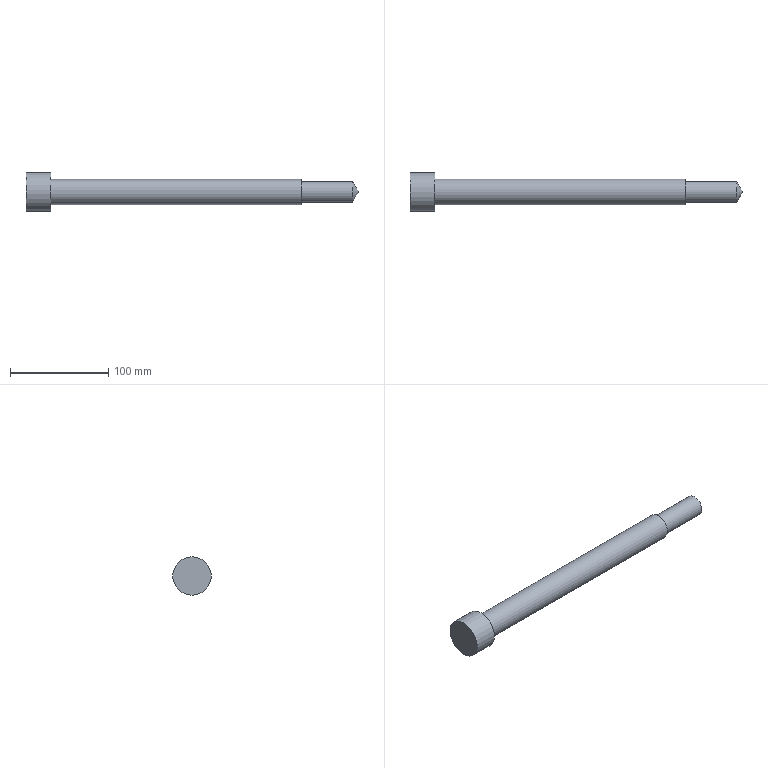Part | STEP file | solid 54 | 1 solid | 8 faces | box 337.5 x 39 x 39 mm | volume 183962 mm3 | plane 4 | cylinder 3 | cone 1 | commonest cylinder face diameters 21 x1 26 x1 39 x1